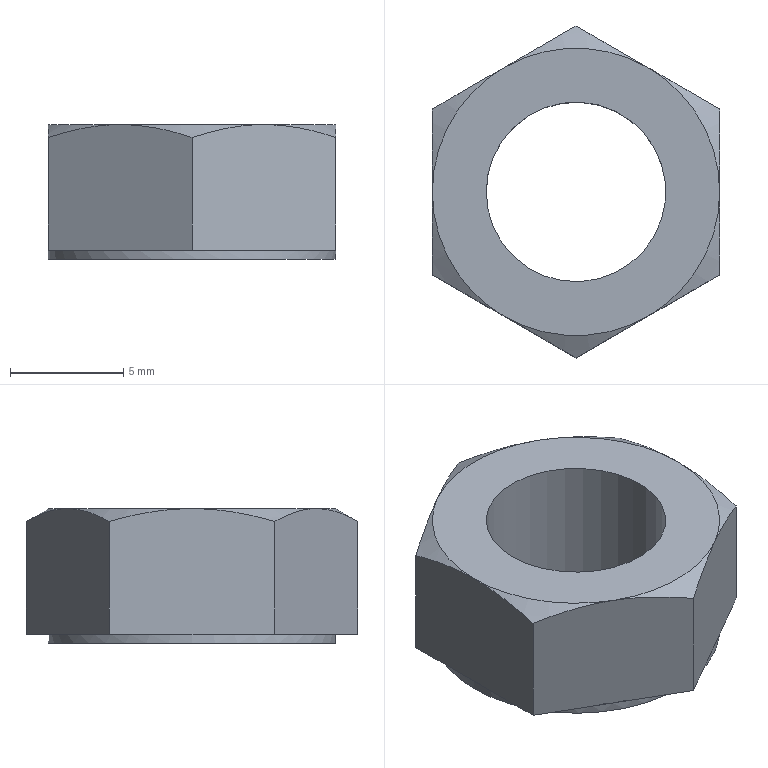Part | NX | features solid 2 | 1 solid | 22 faces | box 12.7 x 14.665 x 5.953 mm | volume 529.41 mm3 | plane 14 | cone 6 | cylinder 2 | commonest cylinder face diameters 7.938 x1 12.7 x1
STEP:
#1=CARTESIAN_POINT('',(3.175,5.499,5.953));
#2=VERTEX_POINT('',#1);
#3=CARTESIAN_POINT('',(0.,7.332,5.386));
#4=VERTEX_POINT('',#3);
#5=CARTESIAN_POINT('',(3.175,5.499,5.953));
#6=CARTESIAN_POINT('',(2.097,6.122,5.953));
#7=CARTESIAN_POINT('',(1.036,6.734,5.731));
#8=CARTESIAN_POINT('',(0.,7.332,5.386));
#9=B_SPLINE_CURVE_WITH_KNOTS('',3,(#5,#6,#7,#8),.UNSPECIFIED.,.F.,.F.,(4,4),(0.00371,0.007406),.UNSPECIFIED.);
#10=EDGE_CURVE('',#2,#4,#9,.T.);
#11=ORIENTED_EDGE('',*,*,#10,.T.);
#12=CARTESIAN_POINT('',(-3.175,5.499,5.953));
#13=VERTEX_POINT('',#12);
#14=CARTESIAN_POINT('',(0.,7.332,5.386));
#15=CARTESIAN_POINT('',(-1.039,6.733,5.732));
#16=CARTESIAN_POINT('',(-2.093,6.124,5.953));
#17=CARTESIAN_POINT('',(-3.175,5.499,5.953));
#18=B_SPLINE_CURVE_WITH_KNOTS('',3,(#14,#15,#16,#17),.UNSPECIFIED.,.F.,.F.,(4,4),(0.000000238,0.00371),.UNSPECIFIED.);
#19=EDGE_CURVE('',#4,#13,#18,.T.);
#20=ORIENTED_EDGE('',*,*,#19,.T.);
#21=CARTESIAN_POINT('',(0.,0.,5.953));
#22=DIRECTION('',(0.,0.,-1.));
#23=DIRECTION('',(-1.,0.,0.));
#24=AXIS2_PLACEMENT_3D('',#21,#22,#23);
#25=CIRCLE('',#24,6.35);
#26=EDGE_CURVE('',#13,#2,#25,.T.);
#27=ORIENTED_EDGE('',*,*,#26,.T.);
#28=EDGE_LOOP('',(#11,#20,#27));
#29=FACE_BOUND('',#28,.T.);
#30=CARTESIAN_POINT('',(0.,0.,5.953));
#31=DIRECTION('',(0.,0.,-1.));
#32=DIRECTION('',(-1.,0.,0.));
#33=AXIS2_PLACEMENT_3D('',#30,#31,#32);
#34=CONICAL_SURFACE('',#33,6.35,1.047);
#35=ADVANCED_FACE('',(#29),#34,.T.);
#36=CARTESIAN_POINT('',(-6.35,0.,5.953));
#37=VERTEX_POINT('',#36);
#38=CARTESIAN_POINT('',(0.,0.,5.953));
#39=DIRECTION('',(0.,0.,-1.));
#40=DIRECTION('',(-1.,0.,0.));
#41=AXIS2_PLACEMENT_3D('',#38,#39,#40);
#42=CIRCLE('',#41,6.35);
#43=EDGE_CURVE('',#37,#13,#42,.T.);
#44=ORIENTED_EDGE('',*,*,#43,.T.);
#45=CARTESIAN_POINT('',(-6.35,3.666,5.386));
#46=VERTEX_POINT('',#45);
#47=CARTESIAN_POINT('',(-3.175,5.499,5.953));
#48=CARTESIAN_POINT('',(-4.253,4.877,5.953));
#49=CARTESIAN_POINT('',(-5.314,4.264,5.731));
#50=CARTESIAN_POINT('',(-6.35,3.666,5.386));
#51=B_SPLINE_CURVE_WITH_KNOTS('',3,(#47,#48,#49,#50),.UNSPECIFIED.,.F.,.F.,(4,4),(0.00371,0.007406),.UNSPECIFIED.);
#52=EDGE_CURVE('',#13,#46,#51,.T.);
#53=ORIENTED_EDGE('',*,*,#52,.T.);
#54=CARTESIAN_POINT('',(-6.35,0.,5.953));
#55=CARTESIAN_POINT('',(-6.35,1.241,5.953));
#56=CARTESIAN_POINT('',(-6.35,2.48,5.728));
#57=CARTESIAN_POINT('',(-6.35,3.666,5.386));
#58=B_SPLINE_CURVE_WITH_KNOTS('',3,(#54,#55,#56,#57),.UNSPECIFIED.,.F.,.F.,(4,4),(0.01045,0.01416),.UNSPECIFIED.);
#59=EDGE_CURVE('',#46,#37,#58,.F.);
#60=ORIENTED_EDGE('',*,*,#59,.T.);
#61=EDGE_LOOP('',(#44,#53,#60));
#62=FACE_BOUND('',#61,.T.);
#63=CARTESIAN_POINT('',(0.,0.,5.953));
#64=DIRECTION('',(0.,0.,-1.));
#65=DIRECTION('',(-1.,0.,0.));
#66=AXIS2_PLACEMENT_3D('',#63,#64,#65);
#67=CONICAL_SURFACE('',#66,6.35,1.047);
#68=ADVANCED_FACE('',(#62),#67,.T.);
#69=CARTESIAN_POINT('',(-3.175,-5.499,5.953));
#70=VERTEX_POINT('',#69);
#71=CARTESIAN_POINT('',(0.,0.,5.953));
#72=DIRECTION('',(0.,0.,-1.));
#73=DIRECTION('',(-1.,0.,0.));
#74=AXIS2_PLACEMENT_3D('',#71,#72,#73);
#75=CIRCLE('',#74,6.35);
#76=EDGE_CURVE('',#70,#37,#75,.T.);
#77=ORIENTED_EDGE('',*,*,#76,.T.);
#78=CARTESIAN_POINT('',(-6.35,-3.666,5.386));
#79=VERTEX_POINT('',#78);
#80=CARTESIAN_POINT('',(-6.35,-3.666,5.386));
#81=CARTESIAN_POINT('',(-6.35,-2.472,5.731));
#82=CARTESIAN_POINT('',(-6.35,-1.24,5.953));
#83=CARTESIAN_POINT('',(-6.35,0.,5.953));
#84=B_SPLINE_CURVE_WITH_KNOTS('',3,(#80,#81,#82,#83),.UNSPECIFIED.,.F.,.F.,(4,4),(0.006737,0.01045),.UNSPECIFIED.);
#85=EDGE_CURVE('',#37,#79,#84,.F.);
#86=ORIENTED_EDGE('',*,*,#85,.T.);
#87=CARTESIAN_POINT('',(-6.35,-3.666,5.386));
#88=CARTESIAN_POINT('',(-5.311,-4.266,5.732));
#89=CARTESIAN_POINT('',(-4.257,-4.875,5.953));
#90=CARTESIAN_POINT('',(-3.175,-5.499,5.953));
#91=B_SPLINE_CURVE_WITH_KNOTS('',3,(#87,#88,#89,#90),.UNSPECIFIED.,.F.,.F.,(4,4),(0.000000238,0.00371),.UNSPECIFIED.);
#92=EDGE_CURVE('',#79,#70,#91,.T.);
#93=ORIENTED_EDGE('',*,*,#92,.T.);
#94=EDGE_LOOP('',(#77,#86,#93));
#95=FACE_BOUND('',#94,.T.);
#96=CARTESIAN_POINT('',(0.,0.,5.953));
#97=DIRECTION('',(0.,0.,-1.));
#98=DIRECTION('',(-1.,0.,0.));
#99=AXIS2_PLACEMENT_3D('',#96,#97,#98);
#100=CONICAL_SURFACE('',#99,6.35,1.047);
#101=ADVANCED_FACE('',(#95),#100,.T.);
#102=CARTESIAN_POINT('',(3.175,-5.499,5.953));
#103=VERTEX_POINT('',#102);
#104=CARTESIAN_POINT('',(0.,0.,5.953));
#105=DIRECTION('',(0.,0.,-1.));
#106=DIRECTION('',(-1.,0.,0.));
#107=AXIS2_PLACEMENT_3D('',#104,#105,#106);
#108=CIRCLE('',#107,6.35);
#109=EDGE_CURVE('',#103,#70,#108,.T.);
#110=ORIENTED_EDGE('',*,*,#109,.T.);
#111=CARTESIAN_POINT('',(0.,-7.332,5.386));
#112=VERTEX_POINT('',#111);
#113=CARTESIAN_POINT('',(-3.175,-5.499,5.953));
#114=CARTESIAN_POINT('',(-2.097,-6.122,5.953));
#115=CARTESIAN_POINT('',(-1.036,-6.734,5.731));
#116=CARTESIAN_POINT('',(0.,-7.332,5.386));
#117=B_SPLINE_CURVE_WITH_KNOTS('',3,(#113,#114,#115,#116),.UNSPECIFIED.,.F.,.F.,(4,4),(0.00371,0.007406),.UNSPECIFIED.);
#118=EDGE_CURVE('',#70,#112,#117,.T.);
#119=ORIENTED_EDGE('',*,*,#118,.T.);
#120=CARTESIAN_POINT('',(0.,-7.332,5.386));
#121=CARTESIAN_POINT('',(1.039,-6.733,5.732));
#122=CARTESIAN_POINT('',(2.093,-6.124,5.953));
#123=CARTESIAN_POINT('',(3.175,-5.499,5.953));
#124=B_SPLINE_CURVE_WITH_KNOTS('',3,(#120,#121,#122,#123),.UNSPECIFIED.,.F.,.F.,(4,4),(0.000000238,0.00371),.UNSPECIFIED.);
#125=EDGE_CURVE('',#112,#103,#124,.T.);
#126=ORIENTED_EDGE('',*,*,#125,.T.);
#127=EDGE_LOOP('',(#110,#119,#126));
#128=FACE_BOUND('',#127,.T.);
#129=CARTESIAN_POINT('',(0.,0.,5.953));
#130=DIRECTION('',(0.,0.,-1.));
#131=DIRECTION('',(-1.,0.,0.));
#132=AXIS2_PLACEMENT_3D('',#129,#130,#131);
#133=CONICAL_SURFACE('',#132,6.35,1.047);
#134=ADVANCED_FACE('',(#128),#133,.T.);
#135=CARTESIAN_POINT('',(6.35,0.,5.953));
#136=VERTEX_POINT('',#135);
#137=CARTESIAN_POINT('',(0.,0.,5.953));
#138=DIRECTION('',(0.,0.,-1.));
#139=DIRECTION('',(-1.,0.,0.));
#140=AXIS2_PLACEMENT_3D('',#137,#138,#139);
#141=CIRCLE('',#140,6.35);
#142=EDGE_CURVE('',#136,#103,#141,.T.);
#143=ORIENTED_EDGE('',*,*,#142,.T.);
#144=CARTESIAN_POINT('',(6.35,-3.666,5.386));
#145=VERTEX_POINT('',#144);
#146=CARTESIAN_POINT('',(3.175,-5.499,5.953));
#147=CARTESIAN_POINT('',(4.253,-4.877,5.953));
#148=CARTESIAN_POINT('',(5.314,-4.264,5.731));
#149=CARTESIAN_POINT('',(6.35,-3.666,5.386));
#150=B_SPLINE_CURVE_WITH_KNOTS('',3,(#146,#147,#148,#149),.UNSPECIFIED.,.F.,.F.,(4,4),(0.00371,0.007406),.UNSPECIFIED.);
#151=EDGE_CURVE('',#103,#145,#150,.T.);
#152=ORIENTED_EDGE('',*,*,#151,.T.);
#153=CARTESIAN_POINT('',(6.35,-3.666,5.386));
#154=CARTESIAN_POINT('',(6.35,-2.472,5.731));
#155=CARTESIAN_POINT('',(6.35,-1.24,5.953));
#156=CARTESIAN_POINT('',(6.35,0.,5.953));
#157=B_SPLINE_CURVE_WITH_KNOTS('',3,(#153,#154,#155,#156),.UNSPECIFIED.,.F.,.F.,(4,4),(0.006737,0.01045),.UNSPECIFIED.);
#158=EDGE_CURVE('',#145,#136,#157,.T.);
#159=ORIENTED_EDGE('',*,*,#158,.T.);
#160=EDGE_LOOP('',(#143,#152,#159));
#161=FACE_BOUND('',#160,.T.);
#162=CARTESIAN_POINT('',(0.,0.,5.953));
#163=DIRECTION('',(0.,0.,-1.));
#164=DIRECTION('',(-1.,0.,0.));
#165=AXIS2_PLACEMENT_3D('',#162,#163,#164);
#166=CONICAL_SURFACE('',#165,6.35,1.047);
#167=ADVANCED_FACE('',(#161),#166,.T.);
#168=CARTESIAN_POINT('',(0.,0.,5.953));
#169=DIRECTION('',(0.,0.,-1.));
#170=DIRECTION('',(-1.,0.,0.));
#171=AXIS2_PLACEMENT_3D('',#168,#169,#170);
#172=CIRCLE('',#171,6.35);
#173=EDGE_CURVE('',#2,#136,#172,.T.);
#174=ORIENTED_EDGE('',*,*,#173,.T.);
#175=CARTESIAN_POINT('',(6.35,3.666,5.386));
#176=VERTEX_POINT('',#175);
#177=CARTESIAN_POINT('',(6.35,0.,5.953));
#178=CARTESIAN_POINT('',(6.35,1.241,5.953));
#179=CARTESIAN_POINT('',(6.35,2.48,5.728));
#180=CARTESIAN_POINT('',(6.35,3.666,5.386));
#181=B_SPLINE_CURVE_WITH_KNOTS('',3,(#177,#178,#179,#180),.UNSPECIFIED.,.F.,.F.,(4,4),(0.01045,0.01416),.UNSPECIFIED.);
#182=EDGE_CURVE('',#136,#176,#181,.T.);
#183=ORIENTED_EDGE('',*,*,#182,.T.);
#184=CARTESIAN_POINT('',(6.35,3.666,5.386));
#185=CARTESIAN_POINT('',(5.311,4.266,5.732));
#186=CARTESIAN_POINT('',(4.257,4.875,5.953));
#187=CARTESIAN_POINT('',(3.175,5.499,5.953));
#188=B_SPLINE_CURVE_WITH_KNOTS('',3,(#184,#185,#186,#187),.UNSPECIFIED.,.F.,.F.,(4,4),(0.000000238,0.00371),.UNSPECIFIED.);
#189=EDGE_CURVE('',#176,#2,#188,.T.);
#190=ORIENTED_EDGE('',*,*,#189,.T.);
#191=EDGE_LOOP('',(#174,#183,#190));
#192=FACE_BOUND('',#191,.T.);
#193=CARTESIAN_POINT('',(0.,0.,5.953));
#194=DIRECTION('',(0.,0.,-1.));
#195=DIRECTION('',(-1.,0.,0.));
#196=AXIS2_PLACEMENT_3D('',#193,#194,#195);
#197=CONICAL_SURFACE('',#196,6.35,1.047);
#198=ADVANCED_FACE('',(#192),#197,.T.);
#199=CARTESIAN_POINT('',(3.175,-5.499,0.4064));
#200=VERTEX_POINT('',#199);
#201=CARTESIAN_POINT('',(0.,-7.332,0.4064));
#202=VERTEX_POINT('',#201);
#203=CARTESIAN_POINT('',(10.319,-1.375,0.4064));
#204=DIRECTION('',(-0.866,-0.5,0.));
#205=VECTOR('',#204,1000.);
#206=LINE('',#203,#205);
#207=EDGE_CURVE('',#200,#202,#206,.T.);
#208=ORIENTED_EDGE('',*,*,#207,.T.);
#209=CARTESIAN_POINT('',(-3.175,-5.499,0.4064));
#210=VERTEX_POINT('',#209);
#211=CARTESIAN_POINT('',(3.969,-9.624,0.4064));
#212=DIRECTION('',(-0.866,0.5,0.));
#213=VECTOR('',#212,1000.);
#214=LINE('',#211,#213);
#215=EDGE_CURVE('',#202,#210,#214,.T.);
#216=ORIENTED_EDGE('',*,*,#215,.T.);
#217=CARTESIAN_POINT('',(0.,0.,0.4064));
#218=DIRECTION('',(0.,0.,-1.));
#219=DIRECTION('',(-1.,0.,0.));
#220=AXIS2_PLACEMENT_3D('',#217,#218,#219);
#221=CIRCLE('',#220,6.35);
#222=EDGE_CURVE('',#200,#210,#221,.T.);
#223=ORIENTED_EDGE('',*,*,#222,.F.);
#224=EDGE_LOOP('',(#208,#216,#223));
#225=FACE_BOUND('',#224,.T.);
#226=CARTESIAN_POINT('',(9.525,0.,0.4064));
#227=DIRECTION('',(0.,0.,1.));
#228=DIRECTION('',(1.,0.,0.));
#229=AXIS2_PLACEMENT_3D('',#226,#227,#228);
#230=PLANE('',#229);
#231=ADVANCED_FACE('',(#225),#230,.F.);
#232=CARTESIAN_POINT('',(-6.35,0.,0.4064));
#233=VERTEX_POINT('',#232);
#234=CARTESIAN_POINT('',(0.,0.,0.4064));
#235=DIRECTION('',(0.,0.,-1.));
#236=DIRECTION('',(-1.,0.,0.));
#237=AXIS2_PLACEMENT_3D('',#234,#235,#236);
#238=CIRCLE('',#237,6.35);
#239=EDGE_CURVE('',#210,#233,#238,.T.);
#240=ORIENTED_EDGE('',*,*,#239,.F.);
#241=CARTESIAN_POINT('',(-6.35,-3.666,0.4064));
#242=VERTEX_POINT('',#241);
#243=CARTESIAN_POINT('',(3.969,-9.624,0.4064));
#244=DIRECTION('',(-0.866,0.5,0.));
#245=VECTOR('',#244,1000.);
#246=LINE('',#243,#245);
#247=EDGE_CURVE('',#210,#242,#246,.T.);
#248=ORIENTED_EDGE('',*,*,#247,.T.);
#249=CARTESIAN_POINT('',(-6.35,0.,0.4064));
#250=DIRECTION('',(0.,1.,0.));
#251=VECTOR('',#250,1000.);
#252=LINE('',#249,#251);
#253=EDGE_CURVE('',#242,#233,#252,.T.);
#254=ORIENTED_EDGE('',*,*,#253,.T.);
#255=EDGE_LOOP('',(#240,#248,#254));
#256=FACE_BOUND('',#255,.T.);
#257=CARTESIAN_POINT('',(9.525,0.,0.4064));
#258=DIRECTION('',(0.,0.,1.));
#259=DIRECTION('',(1.,0.,0.));
#260=AXIS2_PLACEMENT_3D('',#257,#258,#259);
#261=PLANE('',#260);
#262=ADVANCED_FACE('',(#256),#261,.F.);
#263=CARTESIAN_POINT('',(-3.175,5.499,0.4064));
#264=VERTEX_POINT('',#263);
#265=CARTESIAN_POINT('',(0.,0.,0.4064));
#266=DIRECTION('',(0.,0.,-1.));
#267=DIRECTION('',(-1.,0.,0.));
#268=AXIS2_PLACEMENT_3D('',#265,#266,#267);
#269=CIRCLE('',#268,6.35);
#270=EDGE_CURVE('',#233,#264,#269,.T.);
#271=ORIENTED_EDGE('',*,*,#270,.F.);
#272=CARTESIAN_POINT('',(-6.35,3.666,0.4064));
#273=VERTEX_POINT('',#272);
#274=CARTESIAN_POINT('',(-6.35,0.,0.4064));
#275=DIRECTION('',(0.,1.,0.));
#276=VECTOR('',#275,1000.);
#277=LINE('',#274,#276);
#278=EDGE_CURVE('',#233,#273,#277,.T.);
#279=ORIENTED_EDGE('',*,*,#278,.T.);
#280=CARTESIAN_POINT('',(3.969,9.624,0.4064));
#281=DIRECTION('',(0.866,0.5,0.));
#282=VECTOR('',#281,1000.);
#283=LINE('',#280,#282);
#284=EDGE_CURVE('',#273,#264,#283,.T.);
#285=ORIENTED_EDGE('',*,*,#284,.T.);
#286=EDGE_LOOP('',(#271,#279,#285));
#287=FACE_BOUND('',#286,.T.);
#288=CARTESIAN_POINT('',(9.525,0.,0.4064));
#289=DIRECTION('',(0.,0.,1.));
#290=DIRECTION('',(1.,0.,0.));
#291=AXIS2_PLACEMENT_3D('',#288,#289,#290);
#292=PLANE('',#291);
#293=ADVANCED_FACE('',(#287),#292,.F.);
#294=CARTESIAN_POINT('',(6.35,0.,0.4064));
#295=VERTEX_POINT('',#294);
#296=CARTESIAN_POINT('',(6.35,-3.666,0.4064));
#297=VERTEX_POINT('',#296);
#298=CARTESIAN_POINT('',(6.35,0.,0.4064));
#299=DIRECTION('',(0.,-1.,0.));
#300=VECTOR('',#299,1000.);
#301=LINE('',#298,#300);
#302=EDGE_CURVE('',#295,#297,#301,.T.);
#303=ORIENTED_EDGE('',*,*,#302,.T.);
#304=CARTESIAN_POINT('',(10.319,-1.375,0.4064));
#305=DIRECTION('',(-0.866,-0.5,0.));
#306=VECTOR('',#305,1000.);
#307=LINE('',#304,#306);
#308=EDGE_CURVE('',#297,#200,#307,.T.);
#309=ORIENTED_EDGE('',*,*,#308,.T.);
#310=CARTESIAN_POINT('',(0.,0.,0.4064));
#311=DIRECTION('',(0.,0.,-1.));
#312=DIRECTION('',(-1.,0.,0.));
#313=AXIS2_PLACEMENT_3D('',#310,#311,#312);
#314=CIRCLE('',#313,6.35);
#315=EDGE_CURVE('',#295,#200,#314,.T.);
#316=ORIENTED_EDGE('',*,*,#315,.F.);
#317=EDGE_LOOP('',(#303,#309,#316));
#318=FACE_BOUND('',#317,.T.);
#319=CARTESIAN_POINT('',(9.525,0.,0.4064));
#320=DIRECTION('',(0.,0.,1.));
#321=DIRECTION('',(1.,0.,0.));
#322=AXIS2_PLACEMENT_3D('',#319,#320,#321);
#323=PLANE('',#322);
#324=ADVANCED_FACE('',(#318),#323,.F.);
#325=CARTESIAN_POINT('',(3.175,5.499,0.4064));
#326=VERTEX_POINT('',#325);
#327=CARTESIAN_POINT('',(0.,0.,0.4064));
#328=DIRECTION('',(0.,0.,-1.));
#329=DIRECTION('',(-1.,0.,0.));
#330=AXIS2_PLACEMENT_3D('',#327,#328,#329);
#331=CIRCLE('',#330,6.35);
#332=EDGE_CURVE('',#264,#326,#331,.T.);
#333=ORIENTED_EDGE('',*,*,#332,.F.);
#334=CARTESIAN_POINT('',(0.,7.332,0.4064));
#335=VERTEX_POINT('',#334);
#336=CARTESIAN_POINT('',(3.969,9.624,0.4064));
#337=DIRECTION('',(0.866,0.5,0.));
#338=VECTOR('',#337,1000.);
#339=LINE('',#336,#338);
#340=EDGE_CURVE('',#264,#335,#339,.T.);
#341=ORIENTED_EDGE('',*,*,#340,.T.);
#342=CARTESIAN_POINT('',(10.319,1.375,0.4064));
#343=DIRECTION('',(0.866,-0.5,0.));
#344=VECTOR('',#343,1000.);
#345=LINE('',#342,#344);
#346=EDGE_CURVE('',#335,#326,#345,.T.);
#347=ORIENTED_EDGE('',*,*,#346,.T.);
#348=EDGE_LOOP('',(#333,#341,#347));
#349=FACE_BOUND('',#348,.T.);
#350=CARTESIAN_POINT('',(9.525,0.,0.4064));
#351=DIRECTION('',(0.,0.,1.));
#352=DIRECTION('',(1.,0.,0.));
#353=AXIS2_PLACEMENT_3D('',#350,#351,#352);
#354=PLANE('',#353);
#355=ADVANCED_FACE('',(#349),#354,.F.);
#356=CARTESIAN_POINT('',(6.35,3.666,0.4064));
#357=VERTEX_POINT('',#356);
#358=CARTESIAN_POINT('',(10.319,1.375,0.4064));
#359=DIRECTION('',(0.866,-0.5,0.));
#360=VECTOR('',#359,1000.);
#361=LINE('',#358,#360);
#362=EDGE_CURVE('',#326,#357,#361,.T.);
#363=ORIENTED_EDGE('',*,*,#362,.T.);
#364=CARTESIAN_POINT('',(6.35,0.,0.4064));
#365=DIRECTION('',(0.,-1.,0.));
#366=VECTOR('',#365,1000.);
#367=LINE('',#364,#366);
#368=EDGE_CURVE('',#357,#295,#367,.T.);
#369=ORIENTED_EDGE('',*,*,#368,.T.);
#370=CARTESIAN_POINT('',(0.,0.,0.4064));
#371=DIRECTION('',(0.,0.,-1.));
#372=DIRECTION('',(-1.,0.,0.));
#373=AXIS2_PLACEMENT_3D('',#370,#371,#372);
#374=CIRCLE('',#373,6.35);
#375=EDGE_CURVE('',#326,#295,#374,.T.);
#376=ORIENTED_EDGE('',*,*,#375,.F.);
#377=EDGE_LOOP('',(#363,#369,#376));
#378=FACE_BOUND('',#377,.T.);
#379=CARTESIAN_POINT('',(9.525,0.,0.4064));
#380=DIRECTION('',(0.,0.,1.));
#381=DIRECTION('',(1.,0.,0.));
#382=AXIS2_PLACEMENT_3D('',#379,#380,#381);
#383=PLANE('',#382);
#384=ADVANCED_FACE('',(#378),#383,.F.);
#385=ORIENTED_EDGE('',*,*,#43,.F.);
#386=ORIENTED_EDGE('',*,*,#76,.F.);
#387=ORIENTED_EDGE('',*,*,#109,.F.);
#388=ORIENTED_EDGE('',*,*,#142,.F.);
#389=ORIENTED_EDGE('',*,*,#173,.F.);
#390=ORIENTED_EDGE('',*,*,#26,.F.);
#391=EDGE_LOOP('',(#385,#386,#387,#388,#389,#390));
#392=FACE_BOUND('',#391,.T.);
#393=CARTESIAN_POINT('',(-3.969,0.,5.953));
#394=VERTEX_POINT('',#393);
#395=CARTESIAN_POINT('',(0.,0.,5.953));
#396=DIRECTION('',(0.,0.,-1.));
#397=DIRECTION('',(-1.,0.,0.));
#398=AXIS2_PLACEMENT_3D('',#395,#396,#397);
#399=CIRCLE('',#398,3.969);
#400=EDGE_CURVE('',#394,#394,#399,.T.);
#401=ORIENTED_EDGE('',*,*,#400,.T.);
#402=EDGE_LOOP('',(#401));
#403=FACE_BOUND('',#402,.T.);
#404=CARTESIAN_POINT('',(3.969,0.,5.953));
#405=DIRECTION('',(0.,0.,-1.));
#406=DIRECTION('',(-1.,0.,0.));
#407=AXIS2_PLACEMENT_3D('',#404,#405,#406);
#408=PLANE('',#407);
#409=ADVANCED_FACE('',(#392,#403),#408,.F.);
#410=CARTESIAN_POINT('',(-6.35,0.,0.));
#411=VERTEX_POINT('',#410);
#412=CARTESIAN_POINT('',(0.,0.,0.));
#413=DIRECTION('',(0.,0.,-1.));
#414=DIRECTION('',(-1.,0.,0.));
#415=AXIS2_PLACEMENT_3D('',#412,#413,#414);
#416=CIRCLE('',#415,6.35);
#417=EDGE_CURVE('',#411,#411,#416,.T.);
#418=ORIENTED_EDGE('',*,*,#417,.F.);
#419=EDGE_LOOP('',(#418));
#420=FACE_BOUND('',#419,.T.);
#421=ORIENTED_EDGE('',*,*,#270,.T.);
#422=ORIENTED_EDGE('',*,*,#332,.T.);
#423=ORIENTED_EDGE('',*,*,#375,.T.);
#424=ORIENTED_EDGE('',*,*,#315,.T.);
#425=ORIENTED_EDGE('',*,*,#222,.T.);
#426=ORIENTED_EDGE('',*,*,#239,.T.);
#427=EDGE_LOOP('',(#421,#422,#423,#424,#425,#426));
#428=FACE_BOUND('',#427,.T.);
#429=CARTESIAN_POINT('',(0.,0.,0.));
#430=DIRECTION('',(0.,0.,-1.));
#431=DIRECTION('',(-1.,0.,0.));
#432=AXIS2_PLACEMENT_3D('',#429,#430,#431);
#433=CYLINDRICAL_SURFACE('',#432,6.35);
#434=ADVANCED_FACE('',(#420,#428),#433,.T.);
#435=CARTESIAN_POINT('',(-3.969,0.,0.));
#436=VERTEX_POINT('',#435);
#437=CARTESIAN_POINT('',(0.,0.,0.));
#438=DIRECTION('',(0.,0.,-1.));
#439=DIRECTION('',(-1.,0.,0.));
#440=AXIS2_PLACEMENT_3D('',#437,#438,#439);
#441=CIRCLE('',#440,3.969);
#442=EDGE_CURVE('',#436,#436,#441,.T.);
#443=ORIENTED_EDGE('',*,*,#442,.F.);
#444=EDGE_LOOP('',(#443));
#445=FACE_BOUND('',#444,.T.);
#446=ORIENTED_EDGE('',*,*,#417,.T.);
#447=EDGE_LOOP('',(#446));
#448=FACE_BOUND('',#447,.T.);
#449=CARTESIAN_POINT('',(6.35,0.,0.));
#450=DIRECTION('',(0.,0.,1.));
#451=DIRECTION('',(1.,0.,0.));
#452=AXIS2_PLACEMENT_3D('',#449,#450,#451);
#453=PLANE('',#452);
#454=ADVANCED_FACE('',(#445,#448),#453,.F.);
#455=ORIENTED_EDGE('',*,*,#400,.F.);
#456=EDGE_LOOP('',(#455));
#457=FACE_BOUND('',#456,.T.);
#458=ORIENTED_EDGE('',*,*,#442,.T.);
#459=EDGE_LOOP('',(#458));
#460=FACE_BOUND('',#459,.T.);
#461=CARTESIAN_POINT('',(0.,0.,0.));
#462=DIRECTION('',(0.,0.,-1.));
#463=DIRECTION('',(-1.,0.,0.));
#464=AXIS2_PLACEMENT_3D('',#461,#462,#463);
#465=CYLINDRICAL_SURFACE('',#464,3.969);
#466=ADVANCED_FACE('',(#457,#460),#465,.F.);
#467=ORIENTED_EDGE('',*,*,#19,.F.);
#468=CARTESIAN_POINT('',(0.,7.332,6.548));
#469=DIRECTION('',(0.,0.,-1.));
#470=VECTOR('',#469,1000.);
#471=LINE('',#468,#470);
#472=EDGE_CURVE('',#4,#335,#471,.T.);
#473=ORIENTED_EDGE('',*,*,#472,.T.);
#474=ORIENTED_EDGE('',*,*,#340,.F.);
#475=ORIENTED_EDGE('',*,*,#284,.F.);
#476=CARTESIAN_POINT('',(-6.35,3.666,6.548));
#477=DIRECTION('',(0.,0.,-1.));
#478=VECTOR('',#477,1000.);
#479=LINE('',#476,#478);
#480=EDGE_CURVE('',#46,#273,#479,.T.);
#481=ORIENTED_EDGE('',*,*,#480,.F.);
#482=ORIENTED_EDGE('',*,*,#52,.F.);
#483=EDGE_LOOP('',(#467,#473,#474,#475,#481,#482));
#484=FACE_BOUND('',#483,.T.);
#485=CARTESIAN_POINT('',(0.,7.332,6.548));
#486=DIRECTION('',(0.5,-0.866,0.));
#487=DIRECTION('',(0.866,0.5,0.));
#488=AXIS2_PLACEMENT_3D('',#485,#486,#487);
#489=PLANE('',#488);
#490=ADVANCED_FACE('',(#484),#489,.F.);
#491=ORIENTED_EDGE('',*,*,#59,.F.);
#492=ORIENTED_EDGE('',*,*,#480,.T.);
#493=ORIENTED_EDGE('',*,*,#278,.F.);
#494=ORIENTED_EDGE('',*,*,#253,.F.);
#495=CARTESIAN_POINT('',(-6.35,-3.666,6.548));
#496=DIRECTION('',(0.,0.,-1.));
#497=VECTOR('',#496,1000.);
#498=LINE('',#495,#497);
#499=EDGE_CURVE('',#79,#242,#498,.T.);
#500=ORIENTED_EDGE('',*,*,#499,.F.);
#501=ORIENTED_EDGE('',*,*,#85,.F.);
#502=EDGE_LOOP('',(#491,#492,#493,#494,#500,#501));
#503=FACE_BOUND('',#502,.T.);
#504=CARTESIAN_POINT('',(-6.35,3.666,6.548));
#505=DIRECTION('',(1.,0.,0.));
#506=DIRECTION('',(0.,1.,0.));
#507=AXIS2_PLACEMENT_3D('',#504,#505,#506);
#508=PLANE('',#507);
#509=ADVANCED_FACE('',(#503),#508,.F.);
#510=ORIENTED_EDGE('',*,*,#92,.F.);
#511=ORIENTED_EDGE('',*,*,#499,.T.);
#512=ORIENTED_EDGE('',*,*,#247,.F.);
#513=ORIENTED_EDGE('',*,*,#215,.F.);
#514=CARTESIAN_POINT('',(0.,-7.332,6.548));
#515=DIRECTION('',(0.,0.,-1.));
#516=VECTOR('',#515,1000.);
#517=LINE('',#514,#516);
#518=EDGE_CURVE('',#112,#202,#517,.T.);
#519=ORIENTED_EDGE('',*,*,#518,.F.);
#520=ORIENTED_EDGE('',*,*,#118,.F.);
#521=EDGE_LOOP('',(#510,#511,#512,#513,#519,#520));
#522=FACE_BOUND('',#521,.T.);
#523=CARTESIAN_POINT('',(-6.35,-3.666,6.548));
#524=DIRECTION('',(0.5,0.866,0.));
#525=DIRECTION('',(-0.866,0.5,0.));
#526=AXIS2_PLACEMENT_3D('',#523,#524,#525);
#527=PLANE('',#526);
#528=ADVANCED_FACE('',(#522),#527,.F.);
#529=ORIENTED_EDGE('',*,*,#125,.F.);
#530=ORIENTED_EDGE('',*,*,#518,.T.);
#531=ORIENTED_EDGE('',*,*,#207,.F.);
#532=ORIENTED_EDGE('',*,*,#308,.F.);
#533=CARTESIAN_POINT('',(6.35,-3.666,6.548));
#534=DIRECTION('',(0.,0.,-1.));
#535=VECTOR('',#534,1000.);
#536=LINE('',#533,#535);
#537=EDGE_CURVE('',#145,#297,#536,.T.);
#538=ORIENTED_EDGE('',*,*,#537,.F.);
#539=ORIENTED_EDGE('',*,*,#151,.F.);
#540=EDGE_LOOP('',(#529,#530,#531,#532,#538,#539));
#541=FACE_BOUND('',#540,.T.);
#542=CARTESIAN_POINT('',(0.,-7.332,6.548));
#543=DIRECTION('',(-0.5,0.866,0.));
#544=DIRECTION('',(-0.866,-0.5,0.));
#545=AXIS2_PLACEMENT_3D('',#542,#543,#544);
#546=PLANE('',#545);
#547=ADVANCED_FACE('',(#541),#546,.F.);
#548=ORIENTED_EDGE('',*,*,#158,.F.);
#549=ORIENTED_EDGE('',*,*,#537,.T.);
#550=ORIENTED_EDGE('',*,*,#302,.F.);
#551=ORIENTED_EDGE('',*,*,#368,.F.);
#552=CARTESIAN_POINT('',(6.35,3.666,6.548));
#553=DIRECTION('',(0.,0.,-1.));
#554=VECTOR('',#553,1000.);
#555=LINE('',#552,#554);
#556=EDGE_CURVE('',#176,#357,#555,.T.);
#557=ORIENTED_EDGE('',*,*,#556,.F.);
#558=ORIENTED_EDGE('',*,*,#182,.F.);
#559=EDGE_LOOP('',(#548,#549,#550,#551,#557,#558));
#560=FACE_BOUND('',#559,.T.);
#561=CARTESIAN_POINT('',(6.35,-3.666,6.548));
#562=DIRECTION('',(-1.,0.,0.));
#563=DIRECTION('',(0.,-1.,0.));
#564=AXIS2_PLACEMENT_3D('',#561,#562,#563);
#565=PLANE('',#564);
#566=ADVANCED_FACE('',(#560),#565,.F.);
#567=ORIENTED_EDGE('',*,*,#189,.F.);
#568=ORIENTED_EDGE('',*,*,#556,.T.);
#569=ORIENTED_EDGE('',*,*,#362,.F.);
#570=ORIENTED_EDGE('',*,*,#346,.F.);
#571=ORIENTED_EDGE('',*,*,#472,.F.);
#572=ORIENTED_EDGE('',*,*,#10,.F.);
#573=EDGE_LOOP('',(#567,#568,#569,#570,#571,#572));
#574=FACE_BOUND('',#573,.T.);
#575=CARTESIAN_POINT('',(6.35,3.666,6.548));
#576=DIRECTION('',(-0.5,-0.866,0.));
#577=DIRECTION('',(0.866,-0.5,0.));
#578=AXIS2_PLACEMENT_3D('',#575,#576,#577);
#579=PLANE('',#578);
#580=ADVANCED_FACE('',(#574),#579,.F.);
#581=CLOSED_SHELL('',(#35,#68,#101,#134,#167,#198,#231,#262,#293,#324,#355,#384,#409,#434,#454,#466,#490,#509,#528,#547,#566,#580));
#582=MANIFOLD_SOLID_BREP('',#581);
#583=(LENGTH_UNIT()NAMED_UNIT(*)SI_UNIT(.MILLI.,.METRE.));
#584=UNCERTAINTY_MEASURE_WITH_UNIT(LENGTH_MEASURE(0.0508),#583,'','');
#585=(NAMED_UNIT(*)PLANE_ANGLE_UNIT()SI_UNIT($,.RADIAN.));
#586=(NAMED_UNIT(*)SI_UNIT($,.STERADIAN.)SOLID_ANGLE_UNIT());
#587=(GEOMETRIC_REPRESENTATION_CONTEXT(3)GLOBAL_UNCERTAINTY_ASSIGNED_CONTEXT((#584))GLOBAL_UNIT_ASSIGNED_CONTEXT((#583,#585,#586))REPRESENTATION_CONTEXT('',''));
#588=ADVANCED_BREP_SHAPE_REPRESENTATION('',(#582),#587);